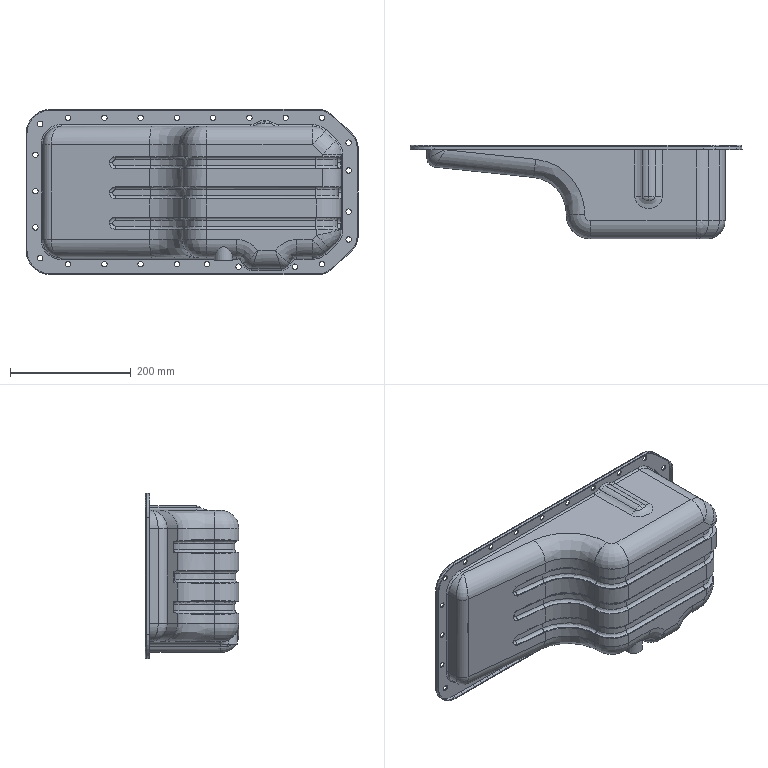Part | SolidWorks | features BaseBody 1 | 1 solid | 456 faces | box 549 x 155 x 273 mm | volume 452407 mm3 | cylinder 242 | spline 110 | plane 72 | torus 32 | commonest cylinder face diameters 9 x50 6 x24 10 x22 57 x20 60 x20 13 x18